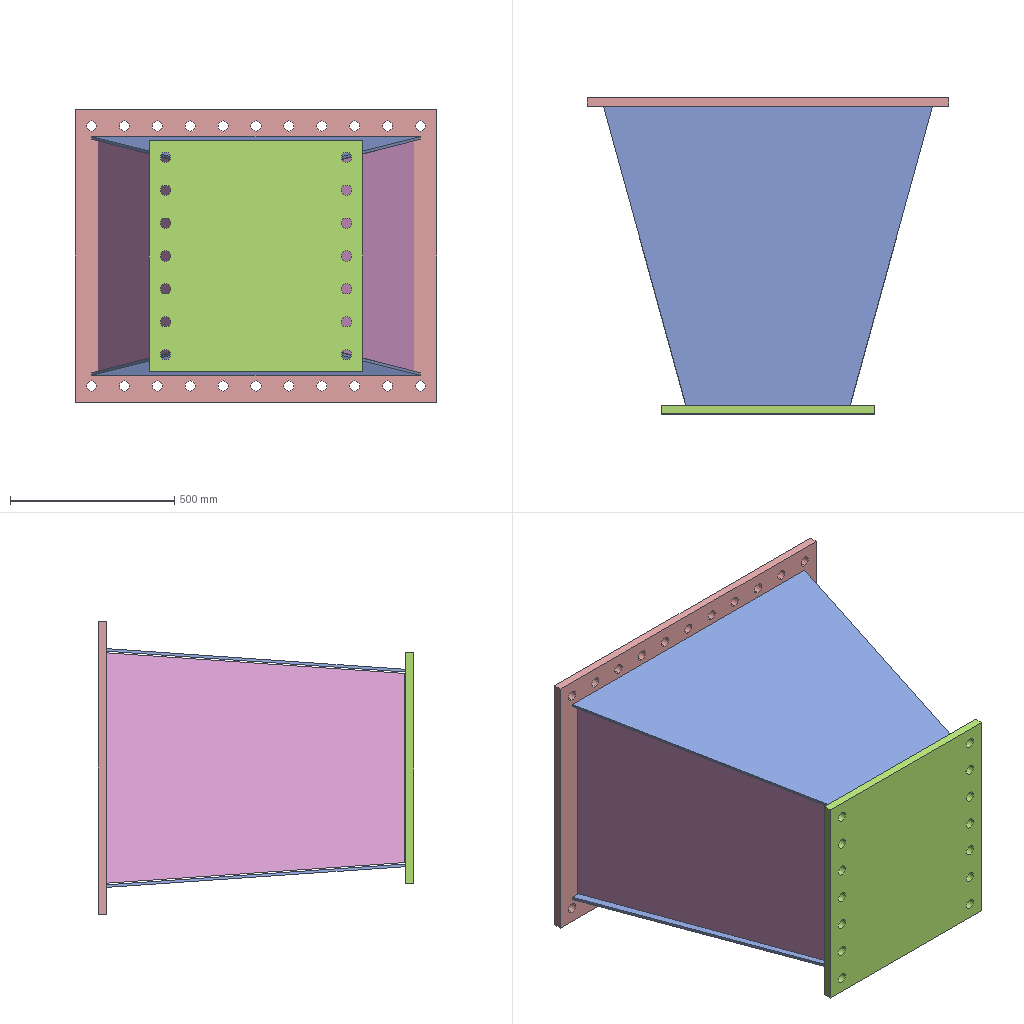Assembly | SolidWorks | 7 different items | 9 placed | box 1100 x 960 x 890 mm
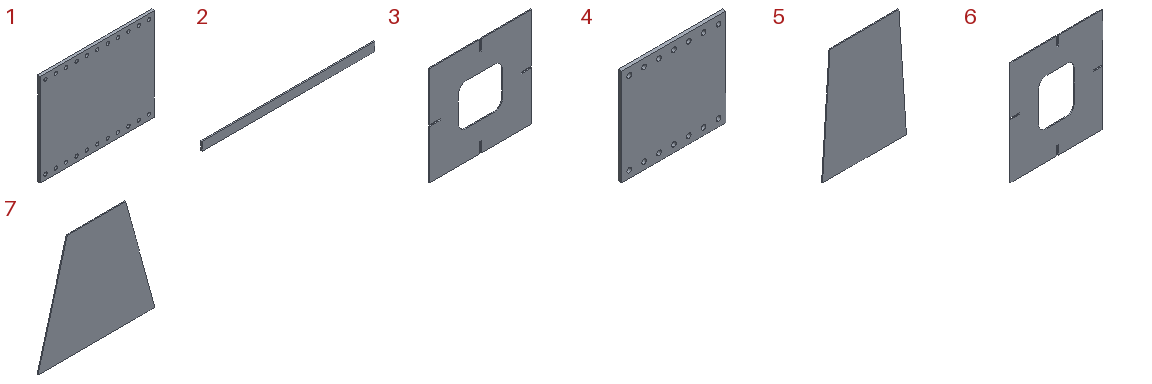Parts list (item | quantity | size | volume | features):
1 | x1 | 1100 x 25 x 890 mm | 24059878 mm3 | features FlatPattern 1, SMBaseFlange 1, SheetMetal 1
2 | x1 | 1200 x 10 x 60 mm | 720000 mm3 | features FlatPattern 1, SMBaseFlange 1, SheetMetal 1
3 | x1 | 620 x 6 x 600 mm | 1824276 mm3 | features FlatPattern 1, SMBaseFlange 1, SheetMetal 1
4 | x1 | 700 x 25 x 650 mm | 11110831 mm3 | features FlatPattern 1, SMBaseFlange 1, SheetMetal 1
5 | x2 | 700 x 8 x 935 mm | 4768500 mm3 | features FlatPattern 1, SMBaseFlange 1, SheetMetal 1
6 | x1 | 645 x 6 x 720 mm | 2313276 mm3 | features FlatPattern 1, SMBaseFlange 1, SheetMetal 1
7 | x2 | 1000 x 8 x 910 mm | 5460000 mm3 | features FlatPattern 1, SMBaseFlange 1, SheetMetal 1
Mates (type | each side: item.copy, entity, surface, feature):
Coincident | 1.1 face plane Base-Flange1 | 7.1 edge
DistanceDim | 1.1 face plane Base-Flange1 | 7.1 edge | 2 times
DistanceDim | 1.1 face plane Base-Flange1 | 4.1 face plane Base-Flange1 | 2 times
DistanceDim | 4.1 face plane Base-Flange1 | 1.1 face plane Base-Flange1
Coincident | 1.1 face plane Base-Flange1 | 5.1 edge
DistanceDim | 1.1 face plane Base-Flange1 | 5.1 edge | 2 times
DistanceDim | 7.2 edge | 4.1 face plane Base-Flange1
PlanarAngleDim | 1.1 face plane Base-Flange1 | 5.2 face plane Base-Flange1
DistanceDim | 1.1 face plane Base-Flange1 | 6.1 face plane Base-Flange1 | 3 times